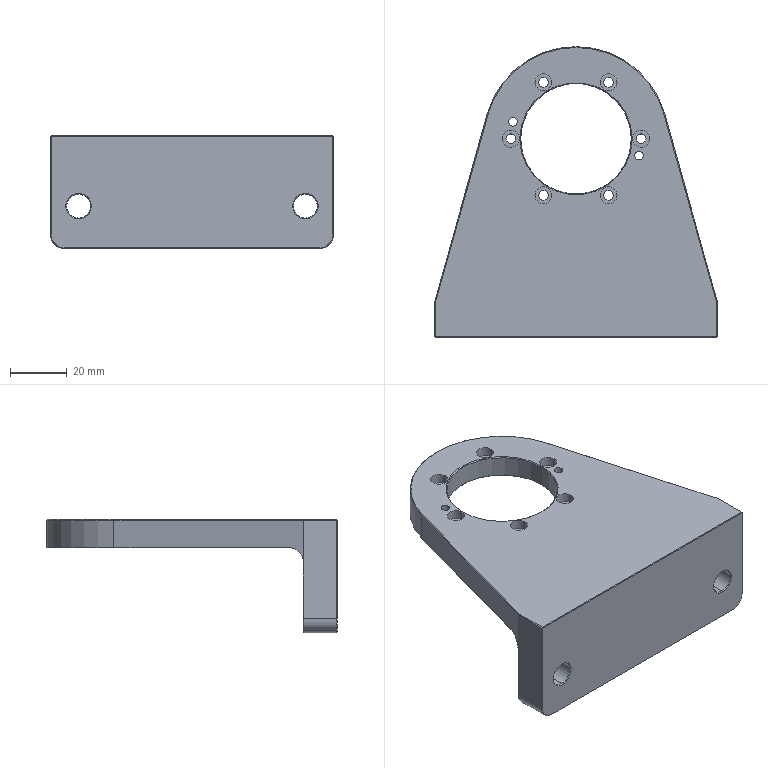Part | 1 solid | 83 faces | box 100 x 102.5 x 40 mm | volume 97654 mm3 | cylinder 40 | plane 26 | cone 17 | commonest cylinder face diameters 3.4 x12 6 x12 3 x4 8.4 x4 10 x3 39 x2